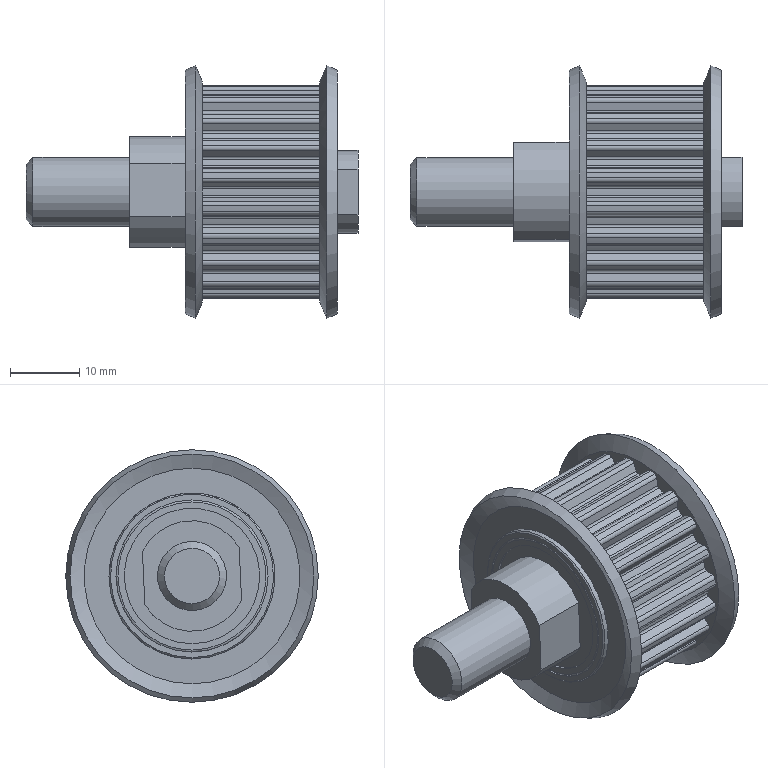Part | NX | 5 solids | 235 faces | box 48 x 36.509 x 36.509 mm | volume 16434 mm3 | cylinder 145 | plane 71 | cone 11 | spline 8 | commonest cylinder face diameters 0.8 x40 1.2 x40 27.4 x20 31 x20 10 x4 13.4 x4